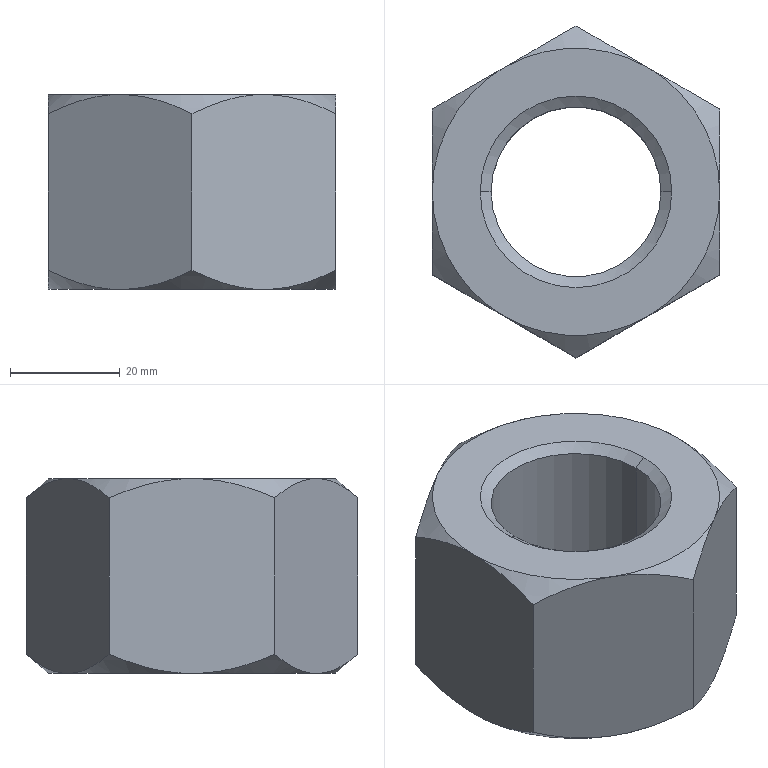Part | SolidWorks | features RevCut 4, Extrusion 1, LPattern 1 | 1 solid | 28 faces | box 52.375 x 60.477 x 35.535 mm | volume 56919 mm3 | cone 16 | plane 8 | cylinder 4 | commonest cylinder face diameters 30.958 x2 34.925 x2
STEP:
#1=CARTESIAN_POINT('',(-0.6875,0.,-1.399));
#2=VERTEX_POINT('',#1);
#3=CARTESIAN_POINT('',(0.6875,0.,-1.399));
#4=VERTEX_POINT('',#3);
#5=CARTESIAN_POINT('',(0.,0.,-1.399));
#6=DIRECTION('',(0.,0.,1.));
#7=DIRECTION('',(-1.,0.,0.));
#8=AXIS2_PLACEMENT_3D('',#5,#6,#7);
#9=CIRCLE('',#8,0.6875);
#10=EDGE_CURVE('',#2,#4,#9,.T.);
#11=ORIENTED_EDGE('',*,*,#10,.F.);
#12=CARTESIAN_POINT('',(-0.6875,0.,-1.398));
#13=VERTEX_POINT('',#12);
#14=CARTESIAN_POINT('',(-0.6875,0.,-0.9857));
#15=DIRECTION('',(0.,0.,1.));
#16=VECTOR('',#15,39.37);
#17=LINE('',#14,#16);
#18=EDGE_CURVE('',#2,#13,#17,.T.);
#19=ORIENTED_EDGE('',*,*,#18,.T.);
#20=CARTESIAN_POINT('',(0.6875,0.,-1.398));
#21=VERTEX_POINT('',#20);
#22=CARTESIAN_POINT('',(0.,0.,-1.398));
#23=DIRECTION('',(0.,0.,1.));
#24=DIRECTION('',(1.,0.,0.));
#25=AXIS2_PLACEMENT_3D('',#22,#23,#24);
#26=CIRCLE('',#25,0.6875);
#27=EDGE_CURVE('',#13,#21,#26,.T.);
#28=ORIENTED_EDGE('',*,*,#27,.T.);
#29=CARTESIAN_POINT('',(0.6875,0.,-0.9857));
#30=DIRECTION('',(0.,0.,1.));
#31=VECTOR('',#30,39.37);
#32=LINE('',#29,#31);
#33=EDGE_CURVE('',#4,#21,#32,.T.);
#34=ORIENTED_EDGE('',*,*,#33,.F.);
#35=EDGE_LOOP('',(#11,#19,#28,#34));
#36=FACE_OUTER_BOUND('',#35,.T.);
#37=CARTESIAN_POINT('',(0.,0.,-0.9857));
#38=DIRECTION('',(0.,0.,1.));
#39=DIRECTION('',(1.,0.,0.));
#40=AXIS2_PLACEMENT_3D('',#37,#38,#39);
#41=CYLINDRICAL_SURFACE('',#40,0.6875);
#42=ADVANCED_FACE('',(#36),#41,.F.);
#43=CARTESIAN_POINT('',(-0.6094,0.,-1.343));
#44=VERTEX_POINT('',#43);
#45=CARTESIAN_POINT('',(0.6094,0.,-1.343));
#46=VERTEX_POINT('',#45);
#47=CARTESIAN_POINT('',(0.,0.,-1.343));
#48=DIRECTION('',(0.,0.,1.));
#49=DIRECTION('',(-1.,0.,0.));
#50=AXIS2_PLACEMENT_3D('',#47,#48,#49);
#51=CIRCLE('',#50,0.6094);
#52=EDGE_CURVE('',#44,#46,#51,.T.);
#53=ORIENTED_EDGE('',*,*,#52,.T.);
#54=CARTESIAN_POINT('',(0.6875,0.,-1.398));
#55=DIRECTION('',(0.8192,0.,-0.5736));
#56=VECTOR('',#55,39.37);
#57=LINE('',#54,#56);
#58=EDGE_CURVE('',#46,#21,#57,.T.);
#59=ORIENTED_EDGE('',*,*,#58,.T.);
#60=ORIENTED_EDGE('',*,*,#27,.F.);
#61=CARTESIAN_POINT('',(-0.6875,0.,-1.398));
#62=DIRECTION('',(-0.8192,0.,-0.5736));
#63=VECTOR('',#62,39.37);
#64=LINE('',#61,#63);
#65=EDGE_CURVE('',#44,#13,#64,.T.);
#66=ORIENTED_EDGE('',*,*,#65,.F.);
#67=EDGE_LOOP('',(#53,#59,#60,#66));
#68=FACE_OUTER_BOUND('',#67,.T.);
#69=CARTESIAN_POINT('',(0.,0.,-1.398));
#70=DIRECTION('',(0.,0.,-1.));
#71=DIRECTION('',(-1.,0.,0.));
#72=AXIS2_PLACEMENT_3D('',#69,#70,#71);
#73=CONICAL_SURFACE('',#72,0.6875,0.9599);
#74=ADVANCED_FACE('',(#68),#73,.F.);
#75=CARTESIAN_POINT('',(0.6094,0.,-0.05469));
#76=VERTEX_POINT('',#75);
#77=CARTESIAN_POINT('',(-0.6094,0.,-0.05469));
#78=VERTEX_POINT('',#77);
#79=CARTESIAN_POINT('',(0.,0.,-0.05469));
#80=DIRECTION('',(0.,0.,-1.));
#81=DIRECTION('',(1.,0.,0.));
#82=AXIS2_PLACEMENT_3D('',#79,#80,#81);
#83=CIRCLE('',#82,0.6094);
#84=EDGE_CURVE('',#76,#78,#83,.T.);
#85=ORIENTED_EDGE('',*,*,#84,.T.);
#86=CARTESIAN_POINT('',(-0.6875,0.,0.));
#87=VERTEX_POINT('',#86);
#88=CARTESIAN_POINT('',(-0.6016,0.,-0.06015));
#89=DIRECTION('',(-0.8192,0.,0.5736));
#90=VECTOR('',#89,39.37);
#91=LINE('',#88,#90);
#92=EDGE_CURVE('',#78,#87,#91,.T.);
#93=ORIENTED_EDGE('',*,*,#92,.T.);
#94=CARTESIAN_POINT('',(0.6875,0.,0.));
#95=VERTEX_POINT('',#94);
#96=CARTESIAN_POINT('',(0.,0.,0.));
#97=DIRECTION('',(0.,0.,1.));
#98=DIRECTION('',(1.,0.,0.));
#99=AXIS2_PLACEMENT_3D('',#96,#97,#98);
#100=CIRCLE('',#99,0.6875);
#101=EDGE_CURVE('',#87,#95,#100,.T.);
#102=ORIENTED_EDGE('',*,*,#101,.T.);
#103=CARTESIAN_POINT('',(0.6016,0.,-0.06015));
#104=DIRECTION('',(0.8192,0.,0.5736));
#105=VECTOR('',#104,39.37);
#106=LINE('',#103,#105);
#107=EDGE_CURVE('',#76,#95,#106,.T.);
#108=ORIENTED_EDGE('',*,*,#107,.F.);
#109=EDGE_LOOP('',(#85,#93,#102,#108));
#110=FACE_OUTER_BOUND('',#109,.T.);
#111=CARTESIAN_POINT('',(0.,0.,-0.06015));
#112=DIRECTION('',(0.,0.,1.));
#113=DIRECTION('',(1.,0.,0.));
#114=AXIS2_PLACEMENT_3D('',#111,#112,#113);
#115=CONICAL_SURFACE('',#114,0.6016,0.9599);
#116=ADVANCED_FACE('',(#110),#115,.F.);
#117=ORIENTED_EDGE('',*,*,#52,.F.);
#118=CARTESIAN_POINT('',(-0.6094,0.,-1.399));
#119=DIRECTION('',(0.,0.,1.));
#120=VECTOR('',#119,39.37);
#121=LINE('',#118,#120);
#122=EDGE_CURVE('',#44,#78,#121,.T.);
#123=ORIENTED_EDGE('',*,*,#122,.T.);
#124=ORIENTED_EDGE('',*,*,#84,.F.);
#125=CARTESIAN_POINT('',(0.6094,0.,-1.399));
#126=DIRECTION('',(0.,0.,1.));
#127=VECTOR('',#126,39.37);
#128=LINE('',#125,#127);
#129=EDGE_CURVE('',#46,#76,#128,.T.);
#130=ORIENTED_EDGE('',*,*,#129,.F.);
#131=EDGE_LOOP('',(#117,#123,#124,#130));
#132=FACE_OUTER_BOUND('',#131,.T.);
#133=CARTESIAN_POINT('',(0.,0.,-1.399));
#134=DIRECTION('',(0.,0.,1.));
#135=DIRECTION('',(1.,0.,0.));
#136=AXIS2_PLACEMENT_3D('',#133,#134,#135);
#137=CYLINDRICAL_SURFACE('',#136,0.6094);
#138=ADVANCED_FACE('',(#132),#137,.F.);
#139=ORIENTED_EDGE('',*,*,#122,.F.);
#140=CARTESIAN_POINT('',(0.,0.,-1.343));
#141=DIRECTION('',(0.,0.,1.));
#142=DIRECTION('',(-1.,0.,0.));
#143=AXIS2_PLACEMENT_3D('',#140,#141,#142);
#144=CIRCLE('',#143,0.6094);
#145=EDGE_CURVE('',#46,#44,#144,.T.);
#146=ORIENTED_EDGE('',*,*,#145,.F.);
#147=ORIENTED_EDGE('',*,*,#129,.T.);
#148=CARTESIAN_POINT('',(0.,0.,-0.05469));
#149=DIRECTION('',(0.,0.,-1.));
#150=DIRECTION('',(1.,0.,0.));
#151=AXIS2_PLACEMENT_3D('',#148,#149,#150);
#152=CIRCLE('',#151,0.6094);
#153=EDGE_CURVE('',#78,#76,#152,.T.);
#154=ORIENTED_EDGE('',*,*,#153,.F.);
#155=EDGE_LOOP('',(#139,#146,#147,#154));
#156=FACE_OUTER_BOUND('',#155,.T.);
#157=CARTESIAN_POINT('',(0.,0.,-1.399));
#158=DIRECTION('',(0.,0.,1.));
#159=DIRECTION('',(1.,0.,0.));
#160=AXIS2_PLACEMENT_3D('',#157,#158,#159);
#161=CYLINDRICAL_SURFACE('',#160,0.6094);
#162=ADVANCED_FACE('',(#156),#161,.F.);
#163=CARTESIAN_POINT('',(-1.031,0.5952,-1.261));
#164=VERTEX_POINT('',#163);
#165=CARTESIAN_POINT('',(-1.031,0.5952,-0.1375));
#166=VERTEX_POINT('',#165);
#167=CARTESIAN_POINT('',(-1.031,0.5952,-1.399));
#168=DIRECTION('',(0.,0.,1.));
#169=VECTOR('',#168,39.37);
#170=LINE('',#167,#169);
#171=EDGE_CURVE('',#164,#166,#170,.T.);
#172=ORIENTED_EDGE('',*,*,#171,.T.);
#173=CARTESIAN_POINT('',(-0.5155,0.8929,0.));
#174=VERTEX_POINT('',#173);
#175=CARTESIAN_POINT('',(-1.031,0.5952,-0.1375));
#176=CARTESIAN_POINT('',(-0.9487,0.6427,-0.09656));
#177=CARTESIAN_POINT('',(-0.8651,0.691,-0.06221));
#178=CARTESIAN_POINT('',(-0.7366,0.7652,-0.02594));
#179=CARTESIAN_POINT('',(-0.6933,0.7902,-0.01642));
#180=CARTESIAN_POINT('',(-0.6273,0.8283,-0.006684));
#181=CARTESIAN_POINT('',(-0.6052,0.8411,-0.0042));
#182=CARTESIAN_POINT('',(-0.5606,0.8668,-0.0008577));
#183=CARTESIAN_POINT('',(-0.5381,0.8798,0.));
#184=CARTESIAN_POINT('',(-0.5155,0.8929,0.));
#185=B_SPLINE_CURVE_WITH_KNOTS('',3,(#175,#176,#177,#178,#179,#180,#181,#182,#183,#184),.UNSPECIFIED.,.F.,.F.,(4,2,2,2,4),(0.000000248,0.007759,0.01164,0.01358,0.01552),.UNSPECIFIED.);
#186=EDGE_CURVE('',#166,#174,#185,.T.);
#187=ORIENTED_EDGE('',*,*,#186,.T.);
#188=CARTESIAN_POINT('',(0.,1.19,-0.1375));
#189=VERTEX_POINT('',#188);
#190=CARTESIAN_POINT('',(-0.5155,0.8929,0.));
#191=CARTESIAN_POINT('',(-0.4257,0.9447,0.));
#192=CARTESIAN_POINT('',(-0.3381,0.9953,-0.01366));
#193=CARTESIAN_POINT('',(-0.2094,1.07,-0.04987));
#194=CARTESIAN_POINT('',(-0.167,1.094,-0.06454));
#195=CARTESIAN_POINT('',(-0.08278,1.143,-0.09813));
#196=CARTESIAN_POINT('',(-0.04107,1.167,-0.1171));
#197=CARTESIAN_POINT('',(0.,1.19,-0.1375));
#198=B_SPLINE_CURVE_WITH_KNOTS('',3,(#190,#191,#192,#193,#194,#195,#196,#197),.UNSPECIFIED.,.F.,.F.,(4,2,2,4),(0.01552,0.02324,0.0271,0.03096),.UNSPECIFIED.);
#199=EDGE_CURVE('',#174,#189,#198,.T.);
#200=ORIENTED_EDGE('',*,*,#199,.T.);
#201=CARTESIAN_POINT('',(0.,1.19,-1.261));
#202=VERTEX_POINT('',#201);
#203=CARTESIAN_POINT('',(0.,1.19,-1.399));
#204=DIRECTION('',(0.,0.,1.));
#205=VECTOR('',#204,39.37);
#206=LINE('',#203,#205);
#207=EDGE_CURVE('',#202,#189,#206,.T.);
#208=ORIENTED_EDGE('',*,*,#207,.F.);
#209=CARTESIAN_POINT('',(-0.5155,0.8929,-1.399));
#210=VERTEX_POINT('',#209);
#211=CARTESIAN_POINT('',(-0.5155,0.8929,-1.399));
#212=CARTESIAN_POINT('',(-0.4257,0.9447,-1.399));
#213=CARTESIAN_POINT('',(-0.3381,0.9953,-1.385));
#214=CARTESIAN_POINT('',(-0.2094,1.07,-1.349));
#215=CARTESIAN_POINT('',(-0.167,1.094,-1.334));
#216=CARTESIAN_POINT('',(-0.08278,1.143,-1.301));
#217=CARTESIAN_POINT('',(-0.04107,1.167,-1.282));
#218=CARTESIAN_POINT('',(0.,1.19,-1.261));
#219=B_SPLINE_CURVE_WITH_KNOTS('',3,(#211,#212,#213,#214,#215,#216,#217,#218),.UNSPECIFIED.,.F.,.F.,(4,2,2,4),(0.01552,0.02324,0.0271,0.03096),.UNSPECIFIED.);
#220=EDGE_CURVE('',#210,#202,#219,.T.);
#221=ORIENTED_EDGE('',*,*,#220,.F.);
#222=CARTESIAN_POINT('',(-1.031,0.5952,-1.261));
#223=CARTESIAN_POINT('',(-0.9487,0.6427,-1.302));
#224=CARTESIAN_POINT('',(-0.8651,0.691,-1.337));
#225=CARTESIAN_POINT('',(-0.7366,0.7652,-1.373));
#226=CARTESIAN_POINT('',(-0.6933,0.7902,-1.383));
#227=CARTESIAN_POINT('',(-0.6273,0.8283,-1.392));
#228=CARTESIAN_POINT('',(-0.6052,0.8411,-1.395));
#229=CARTESIAN_POINT('',(-0.5606,0.8668,-1.398));
#230=CARTESIAN_POINT('',(-0.5381,0.8798,-1.399));
#231=CARTESIAN_POINT('',(-0.5155,0.8929,-1.399));
#232=B_SPLINE_CURVE_WITH_KNOTS('',3,(#222,#223,#224,#225,#226,#227,#228,#229,#230,#231),.UNSPECIFIED.,.F.,.F.,(4,2,2,2,4),(0.000000248,0.007759,0.01164,0.01358,0.01552),.UNSPECIFIED.);
#233=EDGE_CURVE('',#164,#210,#232,.T.);
#234=ORIENTED_EDGE('',*,*,#233,.F.);
#235=EDGE_LOOP('',(#172,#187,#200,#208,#221,#234));
#236=FACE_OUTER_BOUND('',#235,.T.);
#237=CARTESIAN_POINT('',(0.,1.19,-1.399));
#238=DIRECTION('',(-0.5,0.866,0.));
#239=DIRECTION('',(-0.866,-0.5,0.));
#240=AXIS2_PLACEMENT_3D('',#237,#238,#239);
#241=PLANE('',#240);
#242=ADVANCED_FACE('',(#236),#241,.T.);
#243=ORIENTED_EDGE('',*,*,#207,.T.);
#244=CARTESIAN_POINT('',(0.5155,0.8929,0.));
#245=VERTEX_POINT('',#244);
#246=CARTESIAN_POINT('',(0.,1.19,-0.1375));
#247=CARTESIAN_POINT('',(0.08226,1.143,-0.09656));
#248=CARTESIAN_POINT('',(0.1659,1.095,-0.06221));
#249=CARTESIAN_POINT('',(0.2944,1.021,-0.02594));
#250=CARTESIAN_POINT('',(0.3377,0.9955,-0.01642));
#251=CARTESIAN_POINT('',(0.4037,0.9574,-0.006684));
#252=CARTESIAN_POINT('',(0.4258,0.9447,-0.0042));
#253=CARTESIAN_POINT('',(0.4704,0.9189,-0.0008577));
#254=CARTESIAN_POINT('',(0.4929,0.9059,0.));
#255=CARTESIAN_POINT('',(0.5155,0.8929,0.));
#256=B_SPLINE_CURVE_WITH_KNOTS('',3,(#246,#247,#248,#249,#250,#251,#252,#253,#254,#255),.UNSPECIFIED.,.F.,.F.,(4,2,2,2,4),(0.000000248,0.007759,0.01164,0.01358,0.01552),.UNSPECIFIED.);
#257=EDGE_CURVE('',#189,#245,#256,.T.);
#258=ORIENTED_EDGE('',*,*,#257,.T.);
#259=CARTESIAN_POINT('',(1.031,0.5952,-0.1375));
#260=VERTEX_POINT('',#259);
#261=CARTESIAN_POINT('',(0.5155,0.8929,0.));
#262=CARTESIAN_POINT('',(0.6053,0.841,0.));
#263=CARTESIAN_POINT('',(0.6929,0.7905,-0.01366));
#264=CARTESIAN_POINT('',(0.8216,0.7162,-0.04987));
#265=CARTESIAN_POINT('',(0.864,0.6917,-0.06454));
#266=CARTESIAN_POINT('',(0.9482,0.643,-0.09813));
#267=CARTESIAN_POINT('',(0.9899,0.619,-0.1171));
#268=CARTESIAN_POINT('',(1.031,0.5952,-0.1375));
#269=B_SPLINE_CURVE_WITH_KNOTS('',3,(#261,#262,#263,#264,#265,#266,#267,#268),.UNSPECIFIED.,.F.,.F.,(4,2,2,4),(0.01552,0.02324,0.0271,0.03096),.UNSPECIFIED.);
#270=EDGE_CURVE('',#245,#260,#269,.T.);
#271=ORIENTED_EDGE('',*,*,#270,.T.);
#272=CARTESIAN_POINT('',(1.031,0.5952,-1.261));
#273=VERTEX_POINT('',#272);
#274=CARTESIAN_POINT('',(1.031,0.5952,-1.399));
#275=DIRECTION('',(0.,0.,1.));
#276=VECTOR('',#275,39.37);
#277=LINE('',#274,#276);
#278=EDGE_CURVE('',#273,#260,#277,.T.);
#279=ORIENTED_EDGE('',*,*,#278,.F.);
#280=CARTESIAN_POINT('',(0.5155,0.8929,-1.399));
#281=VERTEX_POINT('',#280);
#282=CARTESIAN_POINT('',(0.5155,0.8929,-1.399));
#283=CARTESIAN_POINT('',(0.6053,0.841,-1.399));
#284=CARTESIAN_POINT('',(0.6929,0.7905,-1.385));
#285=CARTESIAN_POINT('',(0.8216,0.7162,-1.349));
#286=CARTESIAN_POINT('',(0.864,0.6917,-1.334));
#287=CARTESIAN_POINT('',(0.9482,0.643,-1.301));
#288=CARTESIAN_POINT('',(0.9899,0.619,-1.282));
#289=CARTESIAN_POINT('',(1.031,0.5952,-1.261));
#290=B_SPLINE_CURVE_WITH_KNOTS('',3,(#282,#283,#284,#285,#286,#287,#288,#289),.UNSPECIFIED.,.F.,.F.,(4,2,2,4),(0.01552,0.02324,0.0271,0.03096),.UNSPECIFIED.);
#291=EDGE_CURVE('',#281,#273,#290,.T.);
#292=ORIENTED_EDGE('',*,*,#291,.F.);
#293=CARTESIAN_POINT('',(0.,1.19,-1.261));
#294=CARTESIAN_POINT('',(0.08226,1.143,-1.302));
#295=CARTESIAN_POINT('',(0.1659,1.095,-1.337));
#296=CARTESIAN_POINT('',(0.2944,1.021,-1.373));
#297=CARTESIAN_POINT('',(0.3377,0.9955,-1.383));
#298=CARTESIAN_POINT('',(0.4037,0.9574,-1.392));
#299=CARTESIAN_POINT('',(0.4258,0.9447,-1.395));
#300=CARTESIAN_POINT('',(0.4704,0.9189,-1.398));
#301=CARTESIAN_POINT('',(0.4929,0.9059,-1.399));
#302=CARTESIAN_POINT('',(0.5155,0.8929,-1.399));
#303=B_SPLINE_CURVE_WITH_KNOTS('',3,(#293,#294,#295,#296,#297,#298,#299,#300,#301,#302),.UNSPECIFIED.,.F.,.F.,(4,2,2,2,4),(0.000000248,0.007759,0.01164,0.01358,0.01552),.UNSPECIFIED.);
#304=EDGE_CURVE('',#202,#281,#303,.T.);
#305=ORIENTED_EDGE('',*,*,#304,.F.);
#306=EDGE_LOOP('',(#243,#258,#271,#279,#292,#305));
#307=FACE_OUTER_BOUND('',#306,.T.);
#308=CARTESIAN_POINT('',(1.031,0.5952,-1.399));
#309=DIRECTION('',(0.5,0.866,0.));
#310=DIRECTION('',(-0.866,0.5,0.));
#311=AXIS2_PLACEMENT_3D('',#308,#309,#310);
#312=PLANE('',#311);
#313=ADVANCED_FACE('',(#307),#312,.T.);
#314=CARTESIAN_POINT('',(1.031,-0.5952,-0.1375));
#315=VERTEX_POINT('',#314);
#316=CARTESIAN_POINT('',(1.031,0.,0.));
#317=VERTEX_POINT('',#316);
#318=CARTESIAN_POINT('',(1.031,-0.5952,-0.1375));
#319=CARTESIAN_POINT('',(1.031,-0.5482,-0.1172));
#320=CARTESIAN_POINT('',(1.031,-0.5005,-0.09843));
#321=CARTESIAN_POINT('',(1.031,-0.4028,-0.06464));
#322=CARTESIAN_POINT('',(1.031,-0.3534,-0.04988));
#323=CARTESIAN_POINT('',(1.031,-0.2044,-0.01356));
#324=CARTESIAN_POINT('',(1.031,-0.1033,0.));
#325=CARTESIAN_POINT('',(1.031,0.,0.));
#326=B_SPLINE_CURVE_WITH_KNOTS('',3,(#318,#319,#320,#321,#322,#323,#324,#325),.UNSPECIFIED.,.F.,.F.,(4,2,2,4),(0.02116,0.02505,0.02893,0.0367),.UNSPECIFIED.);
#327=EDGE_CURVE('',#315,#317,#326,.T.);
#328=ORIENTED_EDGE('',*,*,#327,.F.);
#329=CARTESIAN_POINT('',(1.031,-0.5952,-1.261));
#330=VERTEX_POINT('',#329);
#331=CARTESIAN_POINT('',(1.031,-0.5952,-1.399));
#332=DIRECTION('',(0.,0.,1.));
#333=VECTOR('',#332,39.37);
#334=LINE('',#331,#333);
#335=EDGE_CURVE('',#330,#315,#334,.T.);
#336=ORIENTED_EDGE('',*,*,#335,.F.);
#337=CARTESIAN_POINT('',(1.031,0.,-1.399));
#338=VERTEX_POINT('',#337);
#339=CARTESIAN_POINT('',(1.031,-0.5952,-1.261));
#340=CARTESIAN_POINT('',(1.031,-0.5482,-1.282));
#341=CARTESIAN_POINT('',(1.031,-0.5005,-1.301));
#342=CARTESIAN_POINT('',(1.031,-0.4028,-1.334));
#343=CARTESIAN_POINT('',(1.031,-0.3534,-1.349));
#344=CARTESIAN_POINT('',(1.031,-0.2044,-1.385));
#345=CARTESIAN_POINT('',(1.031,-0.1033,-1.399));
#346=CARTESIAN_POINT('',(1.031,0.,-1.399));
#347=B_SPLINE_CURVE_WITH_KNOTS('',3,(#339,#340,#341,#342,#343,#344,#345,#346),.UNSPECIFIED.,.F.,.F.,(4,2,2,4),(0.02116,0.02505,0.02893,0.0367),.UNSPECIFIED.);
#348=EDGE_CURVE('',#330,#338,#347,.T.);
#349=ORIENTED_EDGE('',*,*,#348,.T.);
#350=CARTESIAN_POINT('',(1.031,0.,-1.399));
#351=CARTESIAN_POINT('',(1.031,0.02574,-1.399));
#352=CARTESIAN_POINT('',(1.031,0.05169,-1.398));
#353=CARTESIAN_POINT('',(1.031,0.1031,-1.395));
#354=CARTESIAN_POINT('',(1.031,0.1287,-1.392));
#355=CARTESIAN_POINT('',(1.031,0.2048,-1.383));
#356=CARTESIAN_POINT('',(1.031,0.2549,-1.373));
#357=CARTESIAN_POINT('',(1.031,0.3541,-1.349));
#358=CARTESIAN_POINT('',(1.031,0.4031,-1.334));
#359=CARTESIAN_POINT('',(1.031,0.476,-1.309));
#360=CARTESIAN_POINT('',(1.031,0.5003,-1.3));
#361=CARTESIAN_POINT('',(1.031,0.5481,-1.281));
#362=CARTESIAN_POINT('',(1.031,0.5718,-1.272));
#363=CARTESIAN_POINT('',(1.031,0.5952,-1.261));
#364=B_SPLINE_CURVE_WITH_KNOTS('',3,(#350,#351,#352,#353,#354,#355,#356,#357,#358,#359,#360,#361,#362,#363),.UNSPECIFIED.,.F.,.F.,(4,2,2,2,2,2,4),(0.0367,0.03864,0.04057,0.04444,0.04831,0.05025,0.05219),.UNSPECIFIED.);
#365=EDGE_CURVE('',#338,#273,#364,.T.);
#366=ORIENTED_EDGE('',*,*,#365,.T.);
#367=ORIENTED_EDGE('',*,*,#278,.T.);
#368=CARTESIAN_POINT('',(1.031,0.,0.));
#369=CARTESIAN_POINT('',(1.031,0.02574,0.));
#370=CARTESIAN_POINT('',(1.031,0.05169,-0.0008418));
#371=CARTESIAN_POINT('',(1.031,0.1031,-0.004161));
#372=CARTESIAN_POINT('',(1.031,0.1287,-0.006633));
#373=CARTESIAN_POINT('',(1.031,0.2048,-0.01633));
#374=CARTESIAN_POINT('',(1.031,0.2549,-0.02585));
#375=CARTESIAN_POINT('',(1.031,0.3541,-0.05007));
#376=CARTESIAN_POINT('',(1.031,0.4031,-0.06476));
#377=CARTESIAN_POINT('',(1.031,0.476,-0.08998));
#378=CARTESIAN_POINT('',(1.031,0.5003,-0.09893));
#379=CARTESIAN_POINT('',(1.031,0.5481,-0.1176));
#380=CARTESIAN_POINT('',(1.031,0.5718,-0.1274));
#381=CARTESIAN_POINT('',(1.031,0.5952,-0.1375));
#382=B_SPLINE_CURVE_WITH_KNOTS('',3,(#368,#369,#370,#371,#372,#373,#374,#375,#376,#377,#378,#379,#380,#381),.UNSPECIFIED.,.F.,.F.,(4,2,2,2,2,2,4),(0.0367,0.03864,0.04057,0.04444,0.04831,0.05025,0.05219),.UNSPECIFIED.);
#383=EDGE_CURVE('',#317,#260,#382,.T.);
#384=ORIENTED_EDGE('',*,*,#383,.F.);
#385=EDGE_LOOP('',(#328,#336,#349,#366,#367,#384));
#386=FACE_OUTER_BOUND('',#385,.T.);
#387=CARTESIAN_POINT('',(1.031,0.5952,-1.399));
#388=DIRECTION('',(-1.,0.,0.));
#389=DIRECTION('',(0.,-1.,0.));
#390=AXIS2_PLACEMENT_3D('',#387,#388,#389);
#391=PLANE('',#390);
#392=ADVANCED_FACE('',(#386),#391,.F.);
#393=ORIENTED_EDGE('',*,*,#335,.T.);
#394=CARTESIAN_POINT('',(0.5155,-0.8929,0.));
#395=VERTEX_POINT('',#394);
#396=CARTESIAN_POINT('',(1.031,-0.5952,-0.1375));
#397=CARTESIAN_POINT('',(0.9487,-0.6427,-0.09656));
#398=CARTESIAN_POINT('',(0.8651,-0.691,-0.06221));
#399=CARTESIAN_POINT('',(0.7366,-0.7652,-0.02594));
#400=CARTESIAN_POINT('',(0.6933,-0.7902,-0.01642));
#401=CARTESIAN_POINT('',(0.6273,-0.8283,-0.006684));
#402=CARTESIAN_POINT('',(0.6052,-0.8411,-0.0042));
#403=CARTESIAN_POINT('',(0.5606,-0.8668,-0.0008577));
#404=CARTESIAN_POINT('',(0.5381,-0.8798,0.));
#405=CARTESIAN_POINT('',(0.5155,-0.8929,0.));
#406=B_SPLINE_CURVE_WITH_KNOTS('',3,(#396,#397,#398,#399,#400,#401,#402,#403,#404,#405),.UNSPECIFIED.,.F.,.F.,(4,2,2,2,4),(0.000000248,0.007759,0.01164,0.01358,0.01552),.UNSPECIFIED.);
#407=EDGE_CURVE('',#315,#395,#406,.T.);
#408=ORIENTED_EDGE('',*,*,#407,.T.);
#409=CARTESIAN_POINT('',(0.,-1.19,-0.1375));
#410=VERTEX_POINT('',#409);
#411=CARTESIAN_POINT('',(0.5155,-0.8929,0.));
#412=CARTESIAN_POINT('',(0.4257,-0.9447,0.));
#413=CARTESIAN_POINT('',(0.3381,-0.9953,-0.01366));
#414=CARTESIAN_POINT('',(0.2094,-1.07,-0.04987));
#415=CARTESIAN_POINT('',(0.167,-1.094,-0.06454));
#416=CARTESIAN_POINT('',(0.08278,-1.143,-0.09813));
#417=CARTESIAN_POINT('',(0.04107,-1.167,-0.1171));
#418=CARTESIAN_POINT('',(0.,-1.19,-0.1375));
#419=B_SPLINE_CURVE_WITH_KNOTS('',3,(#411,#412,#413,#414,#415,#416,#417,#418),.UNSPECIFIED.,.F.,.F.,(4,2,2,4),(0.01552,0.02324,0.0271,0.03096),.UNSPECIFIED.);
#420=EDGE_CURVE('',#395,#410,#419,.T.);
#421=ORIENTED_EDGE('',*,*,#420,.T.);
#422=CARTESIAN_POINT('',(0.,-1.19,-1.261));
#423=VERTEX_POINT('',#422);
#424=CARTESIAN_POINT('',(0.,-1.19,-1.399));
#425=DIRECTION('',(0.,0.,1.));
#426=VECTOR('',#425,39.37);
#427=LINE('',#424,#426);
#428=EDGE_CURVE('',#423,#410,#427,.T.);
#429=ORIENTED_EDGE('',*,*,#428,.F.);
#430=CARTESIAN_POINT('',(0.5155,-0.8929,-1.399));
#431=VERTEX_POINT('',#430);
#432=CARTESIAN_POINT('',(0.5155,-0.8929,-1.399));
#433=CARTESIAN_POINT('',(0.4257,-0.9447,-1.399));
#434=CARTESIAN_POINT('',(0.3381,-0.9953,-1.385));
#435=CARTESIAN_POINT('',(0.2094,-1.07,-1.349));
#436=CARTESIAN_POINT('',(0.167,-1.094,-1.334));
#437=CARTESIAN_POINT('',(0.08278,-1.143,-1.301));
#438=CARTESIAN_POINT('',(0.04107,-1.167,-1.282));
#439=CARTESIAN_POINT('',(0.,-1.19,-1.261));
#440=B_SPLINE_CURVE_WITH_KNOTS('',3,(#432,#433,#434,#435,#436,#437,#438,#439),.UNSPECIFIED.,.F.,.F.,(4,2,2,4),(0.01552,0.02324,0.0271,0.03096),.UNSPECIFIED.);
#441=EDGE_CURVE('',#431,#423,#440,.T.);
#442=ORIENTED_EDGE('',*,*,#441,.F.);
#443=CARTESIAN_POINT('',(1.031,-0.5952,-1.261));
#444=CARTESIAN_POINT('',(0.9487,-0.6427,-1.302));
#445=CARTESIAN_POINT('',(0.8651,-0.691,-1.337));
#446=CARTESIAN_POINT('',(0.7366,-0.7652,-1.373));
#447=CARTESIAN_POINT('',(0.6933,-0.7902,-1.383));
#448=CARTESIAN_POINT('',(0.6273,-0.8283,-1.392));
#449=CARTESIAN_POINT('',(0.6052,-0.8411,-1.395));
#450=CARTESIAN_POINT('',(0.5606,-0.8668,-1.398));
#451=CARTESIAN_POINT('',(0.5381,-0.8798,-1.399));
#452=CARTESIAN_POINT('',(0.5155,-0.8929,-1.399));
#453=B_SPLINE_CURVE_WITH_KNOTS('',3,(#443,#444,#445,#446,#447,#448,#449,#450,#451,#452),.UNSPECIFIED.,.F.,.F.,(4,2,2,2,4),(0.000000248,0.007759,0.01164,0.01358,0.01552),.UNSPECIFIED.);
#454=EDGE_CURVE('',#330,#431,#453,.T.);
#455=ORIENTED_EDGE('',*,*,#454,.F.);
#456=EDGE_LOOP('',(#393,#408,#421,#429,#442,#455));
#457=FACE_OUTER_BOUND('',#456,.T.);
#458=CARTESIAN_POINT('',(0.,-1.19,-1.399));
#459=DIRECTION('',(0.5,-0.866,0.));
#460=DIRECTION('',(0.866,0.5,0.));
#461=AXIS2_PLACEMENT_3D('',#458,#459,#460);
#462=PLANE('',#461);
#463=ADVANCED_FACE('',(#457),#462,.T.);
#464=ORIENTED_EDGE('',*,*,#428,.T.);
#465=CARTESIAN_POINT('',(-0.5155,-0.8929,0.));
#466=VERTEX_POINT('',#465);
#467=CARTESIAN_POINT('',(0.,-1.19,-0.1375));
#468=CARTESIAN_POINT('',(-0.08226,-1.143,-0.09656));
#469=CARTESIAN_POINT('',(-0.1659,-1.095,-0.06221));
#470=CARTESIAN_POINT('',(-0.2944,-1.021,-0.02594));
#471=CARTESIAN_POINT('',(-0.3377,-0.9955,-0.01642));
#472=CARTESIAN_POINT('',(-0.4037,-0.9574,-0.006684));
#473=CARTESIAN_POINT('',(-0.4258,-0.9447,-0.0042));
#474=CARTESIAN_POINT('',(-0.4704,-0.9189,-0.0008577));
#475=CARTESIAN_POINT('',(-0.4929,-0.9059,0.));
#476=CARTESIAN_POINT('',(-0.5155,-0.8929,0.));
#477=B_SPLINE_CURVE_WITH_KNOTS('',3,(#467,#468,#469,#470,#471,#472,#473,#474,#475,#476),.UNSPECIFIED.,.F.,.F.,(4,2,2,2,4),(0.000000248,0.007759,0.01164,0.01358,0.01552),.UNSPECIFIED.);
#478=EDGE_CURVE('',#410,#466,#477,.T.);
#479=ORIENTED_EDGE('',*,*,#478,.T.);
#480=CARTESIAN_POINT('',(-1.031,-0.5952,-0.1375));
#481=VERTEX_POINT('',#480);
#482=CARTESIAN_POINT('',(-0.5155,-0.8929,0.));
#483=CARTESIAN_POINT('',(-0.6053,-0.841,0.));
#484=CARTESIAN_POINT('',(-0.6929,-0.7905,-0.01366));
#485=CARTESIAN_POINT('',(-0.8216,-0.7162,-0.04987));
#486=CARTESIAN_POINT('',(-0.864,-0.6917,-0.06454));
#487=CARTESIAN_POINT('',(-0.9482,-0.643,-0.09813));
#488=CARTESIAN_POINT('',(-0.9899,-0.619,-0.1171));
#489=CARTESIAN_POINT('',(-1.031,-0.5952,-0.1375));
#490=B_SPLINE_CURVE_WITH_KNOTS('',3,(#482,#483,#484,#485,#486,#487,#488,#489),.UNSPECIFIED.,.F.,.F.,(4,2,2,4),(0.01552,0.02324,0.0271,0.03096),.UNSPECIFIED.);
#491=EDGE_CURVE('',#466,#481,#490,.T.);
#492=ORIENTED_EDGE('',*,*,#491,.T.);
#493=CARTESIAN_POINT('',(-1.031,-0.5952,-1.261));
#494=VERTEX_POINT('',#493);
#495=CARTESIAN_POINT('',(-1.031,-0.5952,-1.399));
#496=DIRECTION('',(0.,0.,1.));
#497=VECTOR('',#496,39.37);
#498=LINE('',#495,#497);
#499=EDGE_CURVE('',#494,#481,#498,.T.);
#500=ORIENTED_EDGE('',*,*,#499,.F.);
#501=CARTESIAN_POINT('',(-0.5155,-0.8929,-1.399));
#502=VERTEX_POINT('',#501);
#503=CARTESIAN_POINT('',(-0.5155,-0.8929,-1.399));
#504=CARTESIAN_POINT('',(-0.6053,-0.841,-1.399));
#505=CARTESIAN_POINT('',(-0.6929,-0.7905,-1.385));
#506=CARTESIAN_POINT('',(-0.8216,-0.7162,-1.349));
#507=CARTESIAN_POINT('',(-0.864,-0.6917,-1.334));
#508=CARTESIAN_POINT('',(-0.9482,-0.643,-1.301));
#509=CARTESIAN_POINT('',(-0.9899,-0.619,-1.282));
#510=CARTESIAN_POINT('',(-1.031,-0.5952,-1.261));
#511=B_SPLINE_CURVE_WITH_KNOTS('',3,(#503,#504,#505,#506,#507,#508,#509,#510),.UNSPECIFIED.,.F.,.F.,(4,2,2,4),(0.01552,0.02324,0.0271,0.03096),.UNSPECIFIED.);
#512=EDGE_CURVE('',#502,#494,#511,.T.);
#513=ORIENTED_EDGE('',*,*,#512,.F.);
#514=CARTESIAN_POINT('',(0.,-1.19,-1.261));
#515=CARTESIAN_POINT('',(-0.08226,-1.143,-1.302));
#516=CARTESIAN_POINT('',(-0.1659,-1.095,-1.337));
#517=CARTESIAN_POINT('',(-0.2944,-1.021,-1.373));
#518=CARTESIAN_POINT('',(-0.3377,-0.9955,-1.383));
#519=CARTESIAN_POINT('',(-0.4037,-0.9574,-1.392));
#520=CARTESIAN_POINT('',(-0.4258,-0.9447,-1.395));
#521=CARTESIAN_POINT('',(-0.4704,-0.9189,-1.398));
#522=CARTESIAN_POINT('',(-0.4929,-0.9059,-1.399));
#523=CARTESIAN_POINT('',(-0.5155,-0.8929,-1.399));
#524=B_SPLINE_CURVE_WITH_KNOTS('',3,(#514,#515,#516,#517,#518,#519,#520,#521,#522,#523),.UNSPECIFIED.,.F.,.F.,(4,2,2,2,4),(0.000000248,0.007759,0.01164,0.01358,0.01552),.UNSPECIFIED.);
#525=EDGE_CURVE('',#423,#502,#524,.T.);
#526=ORIENTED_EDGE('',*,*,#525,.F.);
#527=EDGE_LOOP('',(#464,#479,#492,#500,#513,#526));
#528=FACE_OUTER_BOUND('',#527,.T.);
#529=CARTESIAN_POINT('',(-1.031,-0.5952,-1.399));
#530=DIRECTION('',(-0.5,-0.866,0.));
#531=DIRECTION('',(0.866,-0.5,0.));
#532=AXIS2_PLACEMENT_3D('',#529,#530,#531);
#533=PLANE('',#532);
#534=ADVANCED_FACE('',(#528),#533,.T.);
#535=ORIENTED_EDGE('',*,*,#499,.T.);
#536=CARTESIAN_POINT('',(-1.031,0.,0.));
#537=VERTEX_POINT('',#536);
#538=CARTESIAN_POINT('',(-1.031,-0.5952,-0.1375));
#539=CARTESIAN_POINT('',(-1.031,-0.5482,-0.1172));
#540=CARTESIAN_POINT('',(-1.031,-0.5005,-0.09843));
#541=CARTESIAN_POINT('',(-1.031,-0.4028,-0.06464));
#542=CARTESIAN_POINT('',(-1.031,-0.3534,-0.04988));
#543=CARTESIAN_POINT('',(-1.031,-0.2044,-0.01356));
#544=CARTESIAN_POINT('',(-1.031,-0.1033,0.));
#545=CARTESIAN_POINT('',(-1.031,0.,0.));
#546=B_SPLINE_CURVE_WITH_KNOTS('',3,(#538,#539,#540,#541,#542,#543,#544,#545),.UNSPECIFIED.,.F.,.F.,(4,2,2,4),(0.02116,0.02505,0.02893,0.0367),.UNSPECIFIED.);
#547=EDGE_CURVE('',#481,#537,#546,.T.);
#548=ORIENTED_EDGE('',*,*,#547,.T.);
#549=CARTESIAN_POINT('',(-1.031,0.,0.));
#550=CARTESIAN_POINT('',(-1.031,0.02574,0.));
#551=CARTESIAN_POINT('',(-1.031,0.05169,-0.0008418));
#552=CARTESIAN_POINT('',(-1.031,0.1031,-0.004161));
#553=CARTESIAN_POINT('',(-1.031,0.1287,-0.006633));
#554=CARTESIAN_POINT('',(-1.031,0.2048,-0.01633));
#555=CARTESIAN_POINT('',(-1.031,0.2549,-0.02585));
#556=CARTESIAN_POINT('',(-1.031,0.3541,-0.05007));
#557=CARTESIAN_POINT('',(-1.031,0.4031,-0.06476));
#558=CARTESIAN_POINT('',(-1.031,0.476,-0.08998));
#559=CARTESIAN_POINT('',(-1.031,0.5003,-0.09893));
#560=CARTESIAN_POINT('',(-1.031,0.5481,-0.1176));
#561=CARTESIAN_POINT('',(-1.031,0.5718,-0.1274));
#562=CARTESIAN_POINT('',(-1.031,0.5952,-0.1375));
#563=B_SPLINE_CURVE_WITH_KNOTS('',3,(#549,#550,#551,#552,#553,#554,#555,#556,#557,#558,#559,#560,#561,#562),.UNSPECIFIED.,.F.,.F.,(4,2,2,2,2,2,4),(0.0367,0.03864,0.04057,0.04444,0.04831,0.05025,0.05219),.UNSPECIFIED.);
#564=EDGE_CURVE('',#537,#166,#563,.T.);
#565=ORIENTED_EDGE('',*,*,#564,.T.);
#566=ORIENTED_EDGE('',*,*,#171,.F.);
#567=CARTESIAN_POINT('',(-1.031,0.,-1.399));
#568=VERTEX_POINT('',#567);
#569=CARTESIAN_POINT('',(-1.031,0.,-1.399));
#570=CARTESIAN_POINT('',(-1.031,0.02574,-1.399));
#571=CARTESIAN_POINT('',(-1.031,0.05169,-1.398));
#572=CARTESIAN_POINT('',(-1.031,0.1031,-1.395));
#573=CARTESIAN_POINT('',(-1.031,0.1287,-1.392));
#574=CARTESIAN_POINT('',(-1.031,0.2048,-1.383));
#575=CARTESIAN_POINT('',(-1.031,0.2549,-1.373));
#576=CARTESIAN_POINT('',(-1.031,0.3541,-1.349));
#577=CARTESIAN_POINT('',(-1.031,0.4031,-1.334));
#578=CARTESIAN_POINT('',(-1.031,0.476,-1.309));
#579=CARTESIAN_POINT('',(-1.031,0.5003,-1.3));
#580=CARTESIAN_POINT('',(-1.031,0.5481,-1.281));
#581=CARTESIAN_POINT('',(-1.031,0.5718,-1.272));
#582=CARTESIAN_POINT('',(-1.031,0.5952,-1.261));
#583=B_SPLINE_CURVE_WITH_KNOTS('',3,(#569,#570,#571,#572,#573,#574,#575,#576,#577,#578,#579,#580,#581,#582),.UNSPECIFIED.,.F.,.F.,(4,2,2,2,2,2,4),(0.0367,0.03864,0.04057,0.04444,0.04831,0.05025,0.05219),.UNSPECIFIED.);
#584=EDGE_CURVE('',#568,#164,#583,.T.);
#585=ORIENTED_EDGE('',*,*,#584,.F.);
#586=CARTESIAN_POINT('',(-1.031,-0.5952,-1.261));
#587=CARTESIAN_POINT('',(-1.031,-0.5482,-1.282));
#588=CARTESIAN_POINT('',(-1.031,-0.5005,-1.301));
#589=CARTESIAN_POINT('',(-1.031,-0.4028,-1.334));
#590=CARTESIAN_POINT('',(-1.031,-0.3534,-1.349));
#591=CARTESIAN_POINT('',(-1.031,-0.2044,-1.385));
#592=CARTESIAN_POINT('',(-1.031,-0.1033,-1.399));
#593=CARTESIAN_POINT('',(-1.031,0.,-1.399));
#594=B_SPLINE_CURVE_WITH_KNOTS('',3,(#586,#587,#588,#589,#590,#591,#592,#593),.UNSPECIFIED.,.F.,.F.,(4,2,2,4),(0.02116,0.02505,0.02893,0.0367),.UNSPECIFIED.);
#595=EDGE_CURVE('',#494,#568,#594,.T.);
#596=ORIENTED_EDGE('',*,*,#595,.F.);
#597=EDGE_LOOP('',(#535,#548,#565,#566,#585,#596));
#598=FACE_OUTER_BOUND('',#597,.T.);
#599=CARTESIAN_POINT('',(-1.031,0.5952,-1.399));
#600=DIRECTION('',(-1.,0.,0.));
#601=DIRECTION('',(0.,0.,1.));
#602=AXIS2_PLACEMENT_3D('',#599,#600,#601);
#603=PLANE('',#602);
#604=ADVANCED_FACE('',(#598),#603,.T.);
#605=CARTESIAN_POINT('',(0.,0.,0.));
#606=DIRECTION('',(0.,0.,1.));
#607=DIRECTION('',(1.,0.,0.));
#608=AXIS2_PLACEMENT_3D('',#605,#606,#607);
#609=CIRCLE('',#608,0.6875);
#610=EDGE_CURVE('',#95,#87,#609,.T.);
#611=ORIENTED_EDGE('',*,*,#610,.F.);
#612=ORIENTED_EDGE('',*,*,#101,.F.);
#613=EDGE_LOOP('',(#611,#612));
#614=FACE_BOUND('',#613,.T.);
#615=CARTESIAN_POINT('',(0.,0.,0.));
#616=DIRECTION('',(0.,0.,-1.));
#617=DIRECTION('',(-1.,0.,0.));
#618=AXIS2_PLACEMENT_3D('',#615,#616,#617);
#619=CIRCLE('',#618,1.031);
#620=EDGE_CURVE('',#537,#174,#619,.T.);
#621=ORIENTED_EDGE('',*,*,#620,.F.);
#622=CARTESIAN_POINT('',(0.,0.,0.));
#623=DIRECTION('',(0.,0.,-1.));
#624=DIRECTION('',(-1.,0.,0.));
#625=AXIS2_PLACEMENT_3D('',#622,#623,#624);
#626=CIRCLE('',#625,1.031);
#627=EDGE_CURVE('',#466,#537,#626,.T.);
#628=ORIENTED_EDGE('',*,*,#627,.F.);
#629=CARTESIAN_POINT('',(0.,0.,0.));
#630=DIRECTION('',(0.,0.,-1.));
#631=DIRECTION('',(-1.,0.,0.));
#632=AXIS2_PLACEMENT_3D('',#629,#630,#631);
#633=CIRCLE('',#632,1.031);
#634=EDGE_CURVE('',#395,#466,#633,.T.);
#635=ORIENTED_EDGE('',*,*,#634,.F.);
#636=CARTESIAN_POINT('',(0.,0.,0.));
#637=DIRECTION('',(0.,0.,-1.));
#638=DIRECTION('',(-1.,0.,0.));
#639=AXIS2_PLACEMENT_3D('',#636,#637,#638);
#640=CIRCLE('',#639,1.031);
#641=EDGE_CURVE('',#317,#395,#640,.T.);
#642=ORIENTED_EDGE('',*,*,#641,.F.);
#643=CARTESIAN_POINT('',(0.,0.,0.));
#644=DIRECTION('',(0.,0.,1.));
#645=DIRECTION('',(1.,0.,0.));
#646=AXIS2_PLACEMENT_3D('',#643,#644,#645);
#647=CIRCLE('',#646,1.031);
#648=EDGE_CURVE('',#317,#245,#647,.T.);
#649=ORIENTED_EDGE('',*,*,#648,.T.);
#650=CARTESIAN_POINT('',(0.,0.,0.));
#651=DIRECTION('',(0.,0.,-1.));
#652=DIRECTION('',(-1.,0.,0.));
#653=AXIS2_PLACEMENT_3D('',#650,#651,#652);
#654=CIRCLE('',#653,1.031);
#655=EDGE_CURVE('',#174,#245,#654,.T.);
#656=ORIENTED_EDGE('',*,*,#655,.F.);
#657=EDGE_LOOP('',(#621,#628,#635,#642,#649,#656));
#658=FACE_OUTER_BOUND('',#657,.T.);
#659=CARTESIAN_POINT('',(0.,1.19,0.));
#660=DIRECTION('',(0.,0.,-1.));
#661=DIRECTION('',(-1.,0.,0.));
#662=AXIS2_PLACEMENT_3D('',#659,#660,#661);
#663=PLANE('',#662);
#664=ADVANCED_FACE('',(#614,#658),#663,.F.);
#665=CARTESIAN_POINT('',(0.,0.,-1.399));
#666=DIRECTION('',(0.,0.,1.));
#667=DIRECTION('',(-1.,0.,0.));
#668=AXIS2_PLACEMENT_3D('',#665,#666,#667);
#669=CIRCLE('',#668,0.6875);
#670=EDGE_CURVE('',#4,#2,#669,.T.);
#671=ORIENTED_EDGE('',*,*,#670,.T.);
#672=ORIENTED_EDGE('',*,*,#10,.T.);
#673=EDGE_LOOP('',(#671,#672));
#674=FACE_BOUND('',#673,.T.);
#675=CARTESIAN_POINT('',(0.,0.,-1.399));
#676=DIRECTION('',(0.,0.,1.));
#677=DIRECTION('',(-1.,0.,0.));
#678=AXIS2_PLACEMENT_3D('',#675,#676,#677);
#679=CIRCLE('',#678,1.031);
#680=EDGE_CURVE('',#568,#502,#679,.T.);
#681=ORIENTED_EDGE('',*,*,#680,.F.);
#682=CARTESIAN_POINT('',(0.,0.,-1.399));
#683=DIRECTION('',(0.,0.,1.));
#684=DIRECTION('',(-1.,0.,0.));
#685=AXIS2_PLACEMENT_3D('',#682,#683,#684);
#686=CIRCLE('',#685,1.031);
#687=EDGE_CURVE('',#210,#568,#686,.T.);
#688=ORIENTED_EDGE('',*,*,#687,.F.);
#689=CARTESIAN_POINT('',(0.,0.,-1.399));
#690=DIRECTION('',(0.,0.,1.));
#691=DIRECTION('',(-1.,0.,0.));
#692=AXIS2_PLACEMENT_3D('',#689,#690,#691);
#693=CIRCLE('',#692,1.031);
#694=EDGE_CURVE('',#281,#210,#693,.T.);
#695=ORIENTED_EDGE('',*,*,#694,.F.);
#696=CARTESIAN_POINT('',(0.,0.,-1.399));
#697=DIRECTION('',(0.,0.,1.));
#698=DIRECTION('',(1.,0.,0.));
#699=AXIS2_PLACEMENT_3D('',#696,#697,#698);
#700=CIRCLE('',#699,1.031);
#701=EDGE_CURVE('',#338,#281,#700,.T.);
#702=ORIENTED_EDGE('',*,*,#701,.F.);
#703=CARTESIAN_POINT('',(0.,0.,-1.399));
#704=DIRECTION('',(0.,0.,1.));
#705=DIRECTION('',(-1.,0.,0.));
#706=AXIS2_PLACEMENT_3D('',#703,#704,#705);
#707=CIRCLE('',#706,1.031);
#708=EDGE_CURVE('',#431,#338,#707,.T.);
#709=ORIENTED_EDGE('',*,*,#708,.F.);
#710=CARTESIAN_POINT('',(0.,0.,-1.399));
#711=DIRECTION('',(0.,0.,1.));
#712=DIRECTION('',(-1.,0.,0.));
#713=AXIS2_PLACEMENT_3D('',#710,#711,#712);
#714=CIRCLE('',#713,1.031);
#715=EDGE_CURVE('',#502,#431,#714,.T.);
#716=ORIENTED_EDGE('',*,*,#715,.F.);
#717=EDGE_LOOP('',(#681,#688,#695,#702,#709,#716));
#718=FACE_OUTER_BOUND('',#717,.T.);
#719=CARTESIAN_POINT('',(0.,1.19,-1.399));
#720=DIRECTION('',(0.,0.,-1.));
#721=DIRECTION('',(-1.,0.,0.));
#722=AXIS2_PLACEMENT_3D('',#719,#720,#721);
#723=PLANE('',#722);
#724=ADVANCED_FACE('',(#674,#718),#723,.T.);
#725=ORIENTED_EDGE('',*,*,#233,.T.);
#726=ORIENTED_EDGE('',*,*,#687,.T.);
#727=ORIENTED_EDGE('',*,*,#584,.T.);
#728=EDGE_LOOP('',(#725,#726,#727));
#729=FACE_OUTER_BOUND('',#728,.T.);
#730=CARTESIAN_POINT('',(0.,0.,-1.399));
#731=DIRECTION('',(0.,0.,1.));
#732=DIRECTION('',(1.,0.,0.));
#733=AXIS2_PLACEMENT_3D('',#730,#731,#732);
#734=CONICAL_SURFACE('',#733,1.031,0.8593);
#735=ADVANCED_FACE('',(#729),#734,.T.);
#736=ORIENTED_EDGE('',*,*,#220,.T.);
#737=ORIENTED_EDGE('',*,*,#304,.T.);
#738=ORIENTED_EDGE('',*,*,#694,.T.);
#739=EDGE_LOOP('',(#736,#737,#738));
#740=FACE_OUTER_BOUND('',#739,.T.);
#741=CARTESIAN_POINT('',(0.,0.,-1.399));
#742=DIRECTION('',(0.,0.,1.));
#743=DIRECTION('',(1.,0.,0.));
#744=AXIS2_PLACEMENT_3D('',#741,#742,#743);
#745=CONICAL_SURFACE('',#744,1.031,0.8593);
#746=ADVANCED_FACE('',(#740),#745,.T.);
#747=ORIENTED_EDGE('',*,*,#291,.T.);
#748=ORIENTED_EDGE('',*,*,#365,.F.);
#749=ORIENTED_EDGE('',*,*,#701,.T.);
#750=EDGE_LOOP('',(#747,#748,#749));
#751=FACE_OUTER_BOUND('',#750,.T.);
#752=CARTESIAN_POINT('',(0.,0.,-1.399));
#753=DIRECTION('',(0.,0.,1.));
#754=DIRECTION('',(1.,0.,0.));
#755=AXIS2_PLACEMENT_3D('',#752,#753,#754);
#756=CONICAL_SURFACE('',#755,1.031,0.8593);
#757=ADVANCED_FACE('',(#751),#756,.T.);
#758=ORIENTED_EDGE('',*,*,#454,.T.);
#759=ORIENTED_EDGE('',*,*,#708,.T.);
#760=ORIENTED_EDGE('',*,*,#348,.F.);
#761=EDGE_LOOP('',(#758,#759,#760));
#762=FACE_OUTER_BOUND('',#761,.T.);
#763=CARTESIAN_POINT('',(0.,0.,-1.399));
#764=DIRECTION('',(0.,0.,1.));
#765=DIRECTION('',(1.,0.,0.));
#766=AXIS2_PLACEMENT_3D('',#763,#764,#765);
#767=CONICAL_SURFACE('',#766,1.031,0.8593);
#768=ADVANCED_FACE('',(#762),#767,.T.);
#769=ORIENTED_EDGE('',*,*,#441,.T.);
#770=ORIENTED_EDGE('',*,*,#525,.T.);
#771=ORIENTED_EDGE('',*,*,#715,.T.);
#772=EDGE_LOOP('',(#769,#770,#771));
#773=FACE_OUTER_BOUND('',#772,.T.);
#774=CARTESIAN_POINT('',(0.,0.,-1.399));
#775=DIRECTION('',(0.,0.,1.));
#776=DIRECTION('',(1.,0.,0.));
#777=AXIS2_PLACEMENT_3D('',#774,#775,#776);
#778=CONICAL_SURFACE('',#777,1.031,0.8593);
#779=ADVANCED_FACE('',(#773),#778,.T.);
#780=ORIENTED_EDGE('',*,*,#512,.T.);
#781=ORIENTED_EDGE('',*,*,#595,.T.);
#782=ORIENTED_EDGE('',*,*,#680,.T.);
#783=EDGE_LOOP('',(#780,#781,#782));
#784=FACE_OUTER_BOUND('',#783,.T.);
#785=CARTESIAN_POINT('',(0.,0.,-1.399));
#786=DIRECTION('',(0.,0.,1.));
#787=DIRECTION('',(1.,0.,0.));
#788=AXIS2_PLACEMENT_3D('',#785,#786,#787);
#789=CONICAL_SURFACE('',#788,1.031,0.8593);
#790=ADVANCED_FACE('',(#784),#789,.T.);
#791=ORIENTED_EDGE('',*,*,#627,.T.);
#792=ORIENTED_EDGE('',*,*,#547,.F.);
#793=ORIENTED_EDGE('',*,*,#491,.F.);
#794=EDGE_LOOP('',(#791,#792,#793));
#795=FACE_OUTER_BOUND('',#794,.T.);
#796=CARTESIAN_POINT('',(0.,0.,0.));
#797=DIRECTION('',(0.,0.,-1.));
#798=DIRECTION('',(-1.,0.,0.));
#799=AXIS2_PLACEMENT_3D('',#796,#797,#798);
#800=CONICAL_SURFACE('',#799,1.031,0.8593);
#801=ADVANCED_FACE('',(#795),#800,.T.);
#802=ORIENTED_EDGE('',*,*,#634,.T.);
#803=ORIENTED_EDGE('',*,*,#478,.F.);
#804=ORIENTED_EDGE('',*,*,#420,.F.);
#805=EDGE_LOOP('',(#802,#803,#804));
#806=FACE_OUTER_BOUND('',#805,.T.);
#807=CARTESIAN_POINT('',(0.,0.,0.));
#808=DIRECTION('',(0.,0.,-1.));
#809=DIRECTION('',(-1.,0.,0.));
#810=AXIS2_PLACEMENT_3D('',#807,#808,#809);
#811=CONICAL_SURFACE('',#810,1.031,0.8593);
#812=ADVANCED_FACE('',(#806),#811,.T.);
#813=ORIENTED_EDGE('',*,*,#327,.T.);
#814=ORIENTED_EDGE('',*,*,#641,.T.);
#815=ORIENTED_EDGE('',*,*,#407,.F.);
#816=EDGE_LOOP('',(#813,#814,#815));
#817=FACE_OUTER_BOUND('',#816,.T.);
#818=CARTESIAN_POINT('',(0.,0.,0.));
#819=DIRECTION('',(0.,0.,-1.));
#820=DIRECTION('',(-1.,0.,0.));
#821=AXIS2_PLACEMENT_3D('',#818,#819,#820);
#822=CONICAL_SURFACE('',#821,1.031,0.8593);
#823=ADVANCED_FACE('',(#817),#822,.T.);
#824=ORIENTED_EDGE('',*,*,#648,.F.);
#825=ORIENTED_EDGE('',*,*,#383,.T.);
#826=ORIENTED_EDGE('',*,*,#270,.F.);
#827=EDGE_LOOP('',(#824,#825,#826));
#828=FACE_OUTER_BOUND('',#827,.T.);
#829=CARTESIAN_POINT('',(0.,0.,0.));
#830=DIRECTION('',(0.,0.,-1.));
#831=DIRECTION('',(-1.,0.,0.));
#832=AXIS2_PLACEMENT_3D('',#829,#830,#831);
#833=CONICAL_SURFACE('',#832,1.031,0.8593);
#834=ADVANCED_FACE('',(#828),#833,.T.);
#835=ORIENTED_EDGE('',*,*,#655,.T.);
#836=ORIENTED_EDGE('',*,*,#257,.F.);
#837=ORIENTED_EDGE('',*,*,#199,.F.);
#838=EDGE_LOOP('',(#835,#836,#837));
#839=FACE_OUTER_BOUND('',#838,.T.);
#840=CARTESIAN_POINT('',(0.,0.,0.));
#841=DIRECTION('',(0.,0.,-1.));
#842=DIRECTION('',(-1.,0.,0.));
#843=AXIS2_PLACEMENT_3D('',#840,#841,#842);
#844=CONICAL_SURFACE('',#843,1.031,0.8593);
#845=ADVANCED_FACE('',(#839),#844,.T.);
#846=ORIENTED_EDGE('',*,*,#564,.F.);
#847=ORIENTED_EDGE('',*,*,#620,.T.);
#848=ORIENTED_EDGE('',*,*,#186,.F.);
#849=EDGE_LOOP('',(#846,#847,#848));
#850=FACE_OUTER_BOUND('',#849,.T.);
#851=CARTESIAN_POINT('',(0.,0.,0.));
#852=DIRECTION('',(0.,0.,-1.));
#853=DIRECTION('',(-1.,0.,0.));
#854=AXIS2_PLACEMENT_3D('',#851,#852,#853);
#855=CONICAL_SURFACE('',#854,1.031,0.8593);
#856=ADVANCED_FACE('',(#850),#855,.T.);
#857=ORIENTED_EDGE('',*,*,#92,.F.);
#858=ORIENTED_EDGE('',*,*,#153,.T.);
#859=ORIENTED_EDGE('',*,*,#107,.T.);
#860=ORIENTED_EDGE('',*,*,#610,.T.);
#861=EDGE_LOOP('',(#857,#858,#859,#860));
#862=FACE_OUTER_BOUND('',#861,.T.);
#863=CARTESIAN_POINT('',(0.,0.,-0.06015));
#864=DIRECTION('',(0.,0.,1.));
#865=DIRECTION('',(1.,0.,0.));
#866=AXIS2_PLACEMENT_3D('',#863,#864,#865);
#867=CONICAL_SURFACE('',#866,0.6016,0.9599);
#868=ADVANCED_FACE('',(#862),#867,.F.);
#869=ORIENTED_EDGE('',*,*,#58,.F.);
#870=ORIENTED_EDGE('',*,*,#145,.T.);
#871=ORIENTED_EDGE('',*,*,#65,.T.);
#872=CARTESIAN_POINT('',(0.,0.,-1.398));
#873=DIRECTION('',(0.,0.,1.));
#874=DIRECTION('',(1.,0.,0.));
#875=AXIS2_PLACEMENT_3D('',#872,#873,#874);
#876=CIRCLE('',#875,0.6875);
#877=EDGE_CURVE('',#21,#13,#876,.T.);
#878=ORIENTED_EDGE('',*,*,#877,.F.);
#879=EDGE_LOOP('',(#869,#870,#871,#878));
#880=FACE_OUTER_BOUND('',#879,.T.);
#881=CARTESIAN_POINT('',(0.,0.,-1.398));
#882=DIRECTION('',(0.,0.,-1.));
#883=DIRECTION('',(-1.,0.,0.));
#884=AXIS2_PLACEMENT_3D('',#881,#882,#883);
#885=CONICAL_SURFACE('',#884,0.6875,0.9599);
#886=ADVANCED_FACE('',(#880),#885,.F.);
#887=ORIENTED_EDGE('',*,*,#18,.F.);
#888=ORIENTED_EDGE('',*,*,#670,.F.);
#889=ORIENTED_EDGE('',*,*,#33,.T.);
#890=ORIENTED_EDGE('',*,*,#877,.T.);
#891=EDGE_LOOP('',(#887,#888,#889,#890));
#892=FACE_OUTER_BOUND('',#891,.T.);
#893=CARTESIAN_POINT('',(0.,0.,-0.9857));
#894=DIRECTION('',(0.,0.,1.));
#895=DIRECTION('',(1.,0.,0.));
#896=AXIS2_PLACEMENT_3D('',#893,#894,#895);
#897=CYLINDRICAL_SURFACE('',#896,0.6875);
#898=ADVANCED_FACE('',(#892),#897,.F.);
#899=CLOSED_SHELL('',(#42,#74,#116,#138,#162,#242,#313,#392,#463,#534,#604,#664,#724,#735,#746,#757,#768,#779,#790,#801,#812,#823,#834,#845,#856,#868,#886,#898));
#900=MANIFOLD_SOLID_BREP('',#899);
#901=CARTESIAN_POINT('',(0.,0.,0.));
#902=DIRECTION('',(0.,0.,1.));
#903=DIRECTION('',(1.,0.,0.));
#904=AXIS2_PLACEMENT_3D('',#901,#902,#903);
#905=(LENGTH_UNIT()NAMED_UNIT(*)SI_UNIT($,.METRE.));
#906=LENGTH_MEASURE_WITH_UNIT(LENGTH_MEASURE(0.0254),#905);
#907=DIMENSIONAL_EXPONENTS(1.,0.,0.,0.,0.,0.,0.);
#908=(CONVERSION_BASED_UNIT('INCH',#906)LENGTH_UNIT()NAMED_UNIT(#907));
#909=UNCERTAINTY_MEASURE_WITH_UNIT(LENGTH_MEASURE(0.00001),#908,'','');
#910=(NAMED_UNIT(*)PLANE_ANGLE_UNIT()SI_UNIT($,.RADIAN.));
#911=(NAMED_UNIT(*)SI_UNIT($,.STERADIAN.)SOLID_ANGLE_UNIT());
#912=(GEOMETRIC_REPRESENTATION_CONTEXT(3)GLOBAL_UNCERTAINTY_ASSIGNED_CONTEXT((#909))GLOBAL_UNIT_ASSIGNED_CONTEXT((#908,#910,#911))REPRESENTATION_CONTEXT('',''));
#913=ADVANCED_BREP_SHAPE_REPRESENTATION('',(#900,#904),#912);